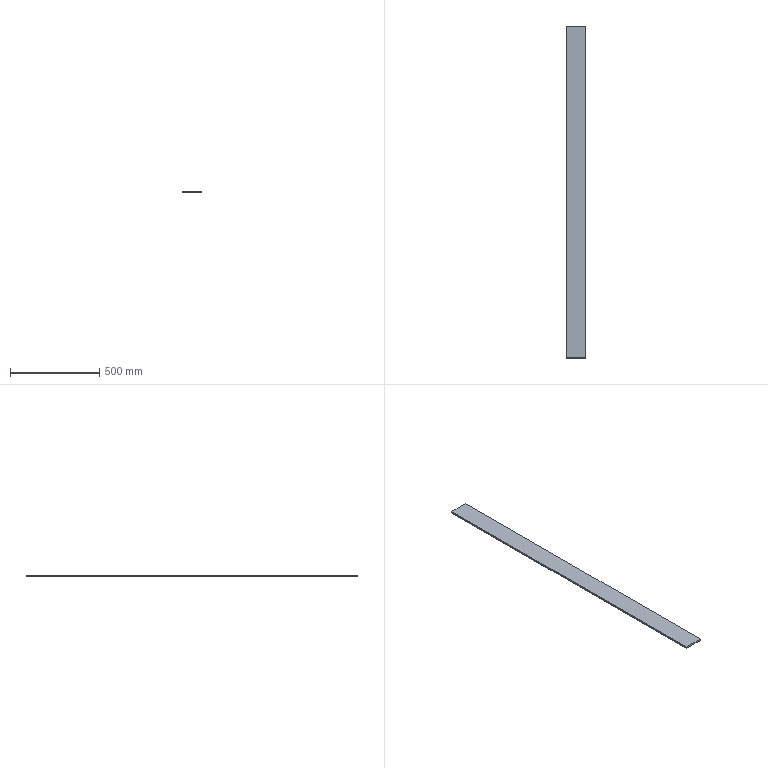Part | STEP file | 02-Steel plate | 1 solid | 6 faces | box 110 x 1860 x 10 mm | volume 2046000 mm3 | plane 6
STEP:
#1=CARTESIAN_POINT('',(0.,0.,0.));
#2=DIRECTION('',(0.,0.,1.));
#3=DIRECTION('',(1.,0.,0.));
#4=AXIS2_PLACEMENT_3D('',#1,#2,#3);
#5=CARTESIAN_POINT('',(0.,0.,0.));
#6=VERTEX_POINT('',#5);
#7=CARTESIAN_POINT('',(0.,-1860.,0.));
#8=VERTEX_POINT('',#7);
#9=CARTESIAN_POINT('',(0.,0.,0.));
#10=DIRECTION('',(0.,-1.,0.));
#11=VECTOR('',#10,1.);
#12=LINE('',#9,#11);
#13=CARTESIAN_POINT('',(0.,0.,10.));
#14=DIRECTION('',(1.,0.,0.));
#15=DIRECTION('',(0.,1.,0.));
#16=AXIS2_PLACEMENT_3D('',#13,#14,#15);
#17=PLANE('',#16);
#18=CARTESIAN_POINT('',(0.,-10.));
#19=DIRECTION('',(-1.,0.));
#20=VECTOR('',#19,1.);
#21=LINE('',#18,#20);
#22=(GEOMETRIC_REPRESENTATION_CONTEXT(2)PARAMETRIC_REPRESENTATION_CONTEXT()REPRESENTATION_CONTEXT('',''));
#23=DEFINITIONAL_REPRESENTATION('',(#21),#22);
#24=PCURVE('',#17,#23);
#25=CARTESIAN_POINT('',(0.,0.,0.));
#26=DIRECTION('',(0.,0.,1.));
#27=DIRECTION('',(1.,0.,0.));
#28=AXIS2_PLACEMENT_3D('',#25,#26,#27);
#29=PLANE('',#28);
#30=CARTESIAN_POINT('',(0.,0.));
#31=DIRECTION('',(0.,-1.));
#32=VECTOR('',#31,1.);
#33=LINE('',#30,#32);
#34=(GEOMETRIC_REPRESENTATION_CONTEXT(2)PARAMETRIC_REPRESENTATION_CONTEXT()REPRESENTATION_CONTEXT('',''));
#35=DEFINITIONAL_REPRESENTATION('',(#33),#34);
#36=PCURVE('',#29,#35);
#37=SURFACE_CURVE('',#12,(#24,#36),.PCURVE_S1.);
#38=EDGE_CURVE('',#6,#8,#37,.T.);
#39=ORIENTED_EDGE('',*,*,#38,.T.);
#40=CARTESIAN_POINT('',(0.,-1860.,10.));
#41=VERTEX_POINT('',#40);
#42=CARTESIAN_POINT('',(0.,-1860.,10.));
#43=DIRECTION('',(0.,0.,-1.));
#44=VECTOR('',#43,1.);
#45=LINE('',#42,#44);
#46=CARTESIAN_POINT('',(-1860.,0.));
#47=DIRECTION('',(0.,-1.));
#48=VECTOR('',#47,1.);
#49=LINE('',#46,#48);
#50=(GEOMETRIC_REPRESENTATION_CONTEXT(2)PARAMETRIC_REPRESENTATION_CONTEXT()REPRESENTATION_CONTEXT('',''));
#51=DEFINITIONAL_REPRESENTATION('',(#49),#50);
#52=PCURVE('',#17,#51);
#53=CARTESIAN_POINT('',(0.,-1860.,10.));
#54=DIRECTION('',(0.,1.,0.));
#55=DIRECTION('',(0.,0.,1.));
#56=AXIS2_PLACEMENT_3D('',#53,#54,#55);
#57=PLANE('',#56);
#58=CARTESIAN_POINT('',(0.,0.));
#59=DIRECTION('',(-1.,0.));
#60=VECTOR('',#59,1.);
#61=LINE('',#58,#60);
#62=(GEOMETRIC_REPRESENTATION_CONTEXT(2)PARAMETRIC_REPRESENTATION_CONTEXT()REPRESENTATION_CONTEXT('',''));
#63=DEFINITIONAL_REPRESENTATION('',(#61),#62);
#64=PCURVE('',#57,#63);
#65=SURFACE_CURVE('',#45,(#52,#64),.PCURVE_S1.);
#66=EDGE_CURVE('',#41,#8,#65,.T.);
#67=ORIENTED_EDGE('',*,*,#66,.F.);
#68=CARTESIAN_POINT('',(0.,0.,10.));
#69=VERTEX_POINT('',#68);
#70=CARTESIAN_POINT('',(0.,0.,10.));
#71=DIRECTION('',(0.,-1.,0.));
#72=VECTOR('',#71,1.);
#73=LINE('',#70,#72);
#74=CARTESIAN_POINT('',(0.,0.));
#75=DIRECTION('',(-1.,0.));
#76=VECTOR('',#75,1.);
#77=LINE('',#74,#76);
#78=(GEOMETRIC_REPRESENTATION_CONTEXT(2)PARAMETRIC_REPRESENTATION_CONTEXT()REPRESENTATION_CONTEXT('',''));
#79=DEFINITIONAL_REPRESENTATION('',(#77),#78);
#80=PCURVE('',#17,#79);
#81=CARTESIAN_POINT('',(0.,0.,10.));
#82=DIRECTION('',(0.,0.,1.));
#83=DIRECTION('',(1.,0.,0.));
#84=AXIS2_PLACEMENT_3D('',#81,#82,#83);
#85=PLANE('',#84);
#86=CARTESIAN_POINT('',(0.,0.));
#87=DIRECTION('',(0.,-1.));
#88=VECTOR('',#87,1.);
#89=LINE('',#86,#88);
#90=(GEOMETRIC_REPRESENTATION_CONTEXT(2)PARAMETRIC_REPRESENTATION_CONTEXT()REPRESENTATION_CONTEXT('',''));
#91=DEFINITIONAL_REPRESENTATION('',(#89),#90);
#92=PCURVE('',#85,#91);
#93=SURFACE_CURVE('',#73,(#80,#92),.PCURVE_S1.);
#94=EDGE_CURVE('',#69,#41,#93,.T.);
#95=ORIENTED_EDGE('',*,*,#94,.F.);
#96=CARTESIAN_POINT('',(0.,0.,10.));
#97=DIRECTION('',(0.,0.,-1.));
#98=VECTOR('',#97,1.);
#99=LINE('',#96,#98);
#100=CARTESIAN_POINT('',(0.,0.));
#101=DIRECTION('',(0.,-1.));
#102=VECTOR('',#101,1.);
#103=LINE('',#100,#102);
#104=(GEOMETRIC_REPRESENTATION_CONTEXT(2)PARAMETRIC_REPRESENTATION_CONTEXT()REPRESENTATION_CONTEXT('',''));
#105=DEFINITIONAL_REPRESENTATION('',(#103),#104);
#106=PCURVE('',#17,#105);
#107=CARTESIAN_POINT('',(0.,0.,10.));
#108=DIRECTION('',(0.,-1.,0.));
#109=DIRECTION('',(0.,0.,-1.));
#110=AXIS2_PLACEMENT_3D('',#107,#108,#109);
#111=PLANE('',#110);
#112=CARTESIAN_POINT('',(0.,0.));
#113=DIRECTION('',(1.,0.));
#114=VECTOR('',#113,1.);
#115=LINE('',#112,#114);
#116=(GEOMETRIC_REPRESENTATION_CONTEXT(2)PARAMETRIC_REPRESENTATION_CONTEXT()REPRESENTATION_CONTEXT('',''));
#117=DEFINITIONAL_REPRESENTATION('',(#115),#116);
#118=PCURVE('',#111,#117);
#119=SURFACE_CURVE('',#99,(#106,#118),.PCURVE_S1.);
#120=EDGE_CURVE('',#69,#6,#119,.T.);
#121=ORIENTED_EDGE('',*,*,#120,.T.);
#122=EDGE_LOOP('',(#39,#67,#95,#121));
#123=FACE_BOUND('',#122,.T.);
#124=ADVANCED_FACE('',(#123),#17,.F.);
#125=CARTESIAN_POINT('',(110.,-1860.,0.));
#126=VERTEX_POINT('',#125);
#127=CARTESIAN_POINT('',(0.,-1860.,0.));
#128=DIRECTION('',(1.,0.,0.));
#129=VECTOR('',#128,1.);
#130=LINE('',#127,#129);
#131=CARTESIAN_POINT('',(-10.,0.));
#132=DIRECTION('',(0.,1.));
#133=VECTOR('',#132,1.);
#134=LINE('',#131,#133);
#135=(GEOMETRIC_REPRESENTATION_CONTEXT(2)PARAMETRIC_REPRESENTATION_CONTEXT()REPRESENTATION_CONTEXT('',''));
#136=DEFINITIONAL_REPRESENTATION('',(#134),#135);
#137=PCURVE('',#57,#136);
#138=CARTESIAN_POINT('',(0.,-1860.));
#139=DIRECTION('',(1.,0.));
#140=VECTOR('',#139,1.);
#141=LINE('',#138,#140);
#142=(GEOMETRIC_REPRESENTATION_CONTEXT(2)PARAMETRIC_REPRESENTATION_CONTEXT()REPRESENTATION_CONTEXT('',''));
#143=DEFINITIONAL_REPRESENTATION('',(#141),#142);
#144=PCURVE('',#29,#143);
#145=SURFACE_CURVE('',#130,(#137,#144),.PCURVE_S1.);
#146=EDGE_CURVE('',#8,#126,#145,.T.);
#147=ORIENTED_EDGE('',*,*,#146,.T.);
#148=CARTESIAN_POINT('',(110.,-1860.,10.));
#149=VERTEX_POINT('',#148);
#150=CARTESIAN_POINT('',(110.,-1860.,10.));
#151=DIRECTION('',(0.,0.,-1.));
#152=VECTOR('',#151,1.);
#153=LINE('',#150,#152);
#154=CARTESIAN_POINT('',(0.,110.));
#155=DIRECTION('',(-1.,0.));
#156=VECTOR('',#155,1.);
#157=LINE('',#154,#156);
#158=(GEOMETRIC_REPRESENTATION_CONTEXT(2)PARAMETRIC_REPRESENTATION_CONTEXT()REPRESENTATION_CONTEXT('',''));
#159=DEFINITIONAL_REPRESENTATION('',(#157),#158);
#160=PCURVE('',#57,#159);
#161=CARTESIAN_POINT('',(110.,0.,10.));
#162=DIRECTION('',(-1.,0.,0.));
#163=DIRECTION('',(0.,-1.,0.));
#164=AXIS2_PLACEMENT_3D('',#161,#162,#163);
#165=PLANE('',#164);
#166=CARTESIAN_POINT('',(1860.,0.));
#167=DIRECTION('',(0.,-1.));
#168=VECTOR('',#167,1.);
#169=LINE('',#166,#168);
#170=(GEOMETRIC_REPRESENTATION_CONTEXT(2)PARAMETRIC_REPRESENTATION_CONTEXT()REPRESENTATION_CONTEXT('',''));
#171=DEFINITIONAL_REPRESENTATION('',(#169),#170);
#172=PCURVE('',#165,#171);
#173=SURFACE_CURVE('',#153,(#160,#172),.PCURVE_S1.);
#174=EDGE_CURVE('',#149,#126,#173,.T.);
#175=ORIENTED_EDGE('',*,*,#174,.F.);
#176=CARTESIAN_POINT('',(0.,-1860.,10.));
#177=DIRECTION('',(1.,0.,0.));
#178=VECTOR('',#177,1.);
#179=LINE('',#176,#178);
#180=CARTESIAN_POINT('',(0.,0.));
#181=DIRECTION('',(0.,1.));
#182=VECTOR('',#181,1.);
#183=LINE('',#180,#182);
#184=(GEOMETRIC_REPRESENTATION_CONTEXT(2)PARAMETRIC_REPRESENTATION_CONTEXT()REPRESENTATION_CONTEXT('',''));
#185=DEFINITIONAL_REPRESENTATION('',(#183),#184);
#186=PCURVE('',#57,#185);
#187=CARTESIAN_POINT('',(0.,-1860.));
#188=DIRECTION('',(1.,0.));
#189=VECTOR('',#188,1.);
#190=LINE('',#187,#189);
#191=(GEOMETRIC_REPRESENTATION_CONTEXT(2)PARAMETRIC_REPRESENTATION_CONTEXT()REPRESENTATION_CONTEXT('',''));
#192=DEFINITIONAL_REPRESENTATION('',(#190),#191);
#193=PCURVE('',#85,#192);
#194=SURFACE_CURVE('',#179,(#186,#193),.PCURVE_S1.);
#195=EDGE_CURVE('',#41,#149,#194,.T.);
#196=ORIENTED_EDGE('',*,*,#195,.F.);
#197=ORIENTED_EDGE('',*,*,#66,.T.);
#198=EDGE_LOOP('',(#147,#175,#196,#197));
#199=FACE_BOUND('',#198,.T.);
#200=ADVANCED_FACE('',(#199),#57,.F.);
#201=CARTESIAN_POINT('',(110.,0.,0.));
#202=VERTEX_POINT('',#201);
#203=CARTESIAN_POINT('',(110.,0.,0.));
#204=DIRECTION('',(0.,1.,0.));
#205=VECTOR('',#204,1.);
#206=LINE('',#203,#205);
#207=CARTESIAN_POINT('',(0.,-10.));
#208=DIRECTION('',(-1.,0.));
#209=VECTOR('',#208,1.);
#210=LINE('',#207,#209);
#211=(GEOMETRIC_REPRESENTATION_CONTEXT(2)PARAMETRIC_REPRESENTATION_CONTEXT()REPRESENTATION_CONTEXT('',''));
#212=DEFINITIONAL_REPRESENTATION('',(#210),#211);
#213=PCURVE('',#165,#212);
#214=CARTESIAN_POINT('',(110.,0.));
#215=DIRECTION('',(0.,1.));
#216=VECTOR('',#215,1.);
#217=LINE('',#214,#216);
#218=(GEOMETRIC_REPRESENTATION_CONTEXT(2)PARAMETRIC_REPRESENTATION_CONTEXT()REPRESENTATION_CONTEXT('',''));
#219=DEFINITIONAL_REPRESENTATION('',(#217),#218);
#220=PCURVE('',#29,#219);
#221=SURFACE_CURVE('',#206,(#213,#220),.PCURVE_S1.);
#222=EDGE_CURVE('',#126,#202,#221,.T.);
#223=ORIENTED_EDGE('',*,*,#222,.T.);
#224=CARTESIAN_POINT('',(110.,0.,10.));
#225=VERTEX_POINT('',#224);
#226=CARTESIAN_POINT('',(110.,0.,10.));
#227=DIRECTION('',(0.,0.,-1.));
#228=VECTOR('',#227,1.);
#229=LINE('',#226,#228);
#230=CARTESIAN_POINT('',(0.,0.));
#231=DIRECTION('',(0.,-1.));
#232=VECTOR('',#231,1.);
#233=LINE('',#230,#232);
#234=(GEOMETRIC_REPRESENTATION_CONTEXT(2)PARAMETRIC_REPRESENTATION_CONTEXT()REPRESENTATION_CONTEXT('',''));
#235=DEFINITIONAL_REPRESENTATION('',(#233),#234);
#236=PCURVE('',#165,#235);
#237=CARTESIAN_POINT('',(0.,110.));
#238=DIRECTION('',(1.,0.));
#239=VECTOR('',#238,1.);
#240=LINE('',#237,#239);
#241=(GEOMETRIC_REPRESENTATION_CONTEXT(2)PARAMETRIC_REPRESENTATION_CONTEXT()REPRESENTATION_CONTEXT('',''));
#242=DEFINITIONAL_REPRESENTATION('',(#240),#241);
#243=PCURVE('',#111,#242);
#244=SURFACE_CURVE('',#229,(#236,#243),.PCURVE_S1.);
#245=EDGE_CURVE('',#225,#202,#244,.T.);
#246=ORIENTED_EDGE('',*,*,#245,.F.);
#247=CARTESIAN_POINT('',(110.,0.,10.));
#248=DIRECTION('',(0.,1.,0.));
#249=VECTOR('',#248,1.);
#250=LINE('',#247,#249);
#251=CARTESIAN_POINT('',(0.,0.));
#252=DIRECTION('',(-1.,0.));
#253=VECTOR('',#252,1.);
#254=LINE('',#251,#253);
#255=(GEOMETRIC_REPRESENTATION_CONTEXT(2)PARAMETRIC_REPRESENTATION_CONTEXT()REPRESENTATION_CONTEXT('',''));
#256=DEFINITIONAL_REPRESENTATION('',(#254),#255);
#257=PCURVE('',#165,#256);
#258=CARTESIAN_POINT('',(110.,0.));
#259=DIRECTION('',(0.,1.));
#260=VECTOR('',#259,1.);
#261=LINE('',#258,#260);
#262=(GEOMETRIC_REPRESENTATION_CONTEXT(2)PARAMETRIC_REPRESENTATION_CONTEXT()REPRESENTATION_CONTEXT('',''));
#263=DEFINITIONAL_REPRESENTATION('',(#261),#262);
#264=PCURVE('',#85,#263);
#265=SURFACE_CURVE('',#250,(#257,#264),.PCURVE_S1.);
#266=EDGE_CURVE('',#149,#225,#265,.T.);
#267=ORIENTED_EDGE('',*,*,#266,.F.);
#268=ORIENTED_EDGE('',*,*,#174,.T.);
#269=EDGE_LOOP('',(#223,#246,#267,#268));
#270=FACE_BOUND('',#269,.T.);
#271=ADVANCED_FACE('',(#270),#165,.F.);
#272=CARTESIAN_POINT('',(0.,0.,0.));
#273=DIRECTION('',(-1.,0.,0.));
#274=VECTOR('',#273,1.);
#275=LINE('',#272,#274);
#276=CARTESIAN_POINT('',(10.,0.));
#277=DIRECTION('',(0.,-1.));
#278=VECTOR('',#277,1.);
#279=LINE('',#276,#278);
#280=(GEOMETRIC_REPRESENTATION_CONTEXT(2)PARAMETRIC_REPRESENTATION_CONTEXT()REPRESENTATION_CONTEXT('',''));
#281=DEFINITIONAL_REPRESENTATION('',(#279),#280);
#282=PCURVE('',#111,#281);
#283=CARTESIAN_POINT('',(0.,0.));
#284=DIRECTION('',(-1.,0.));
#285=VECTOR('',#284,1.);
#286=LINE('',#283,#285);
#287=(GEOMETRIC_REPRESENTATION_CONTEXT(2)PARAMETRIC_REPRESENTATION_CONTEXT()REPRESENTATION_CONTEXT('',''));
#288=DEFINITIONAL_REPRESENTATION('',(#286),#287);
#289=PCURVE('',#29,#288);
#290=SURFACE_CURVE('',#275,(#282,#289),.PCURVE_S1.);
#291=EDGE_CURVE('',#202,#6,#290,.T.);
#292=ORIENTED_EDGE('',*,*,#291,.T.);
#293=ORIENTED_EDGE('',*,*,#120,.F.);
#294=CARTESIAN_POINT('',(0.,0.,10.));
#295=DIRECTION('',(-1.,0.,0.));
#296=VECTOR('',#295,1.);
#297=LINE('',#294,#296);
#298=CARTESIAN_POINT('',(0.,0.));
#299=DIRECTION('',(0.,-1.));
#300=VECTOR('',#299,1.);
#301=LINE('',#298,#300);
#302=(GEOMETRIC_REPRESENTATION_CONTEXT(2)PARAMETRIC_REPRESENTATION_CONTEXT()REPRESENTATION_CONTEXT('',''));
#303=DEFINITIONAL_REPRESENTATION('',(#301),#302);
#304=PCURVE('',#111,#303);
#305=CARTESIAN_POINT('',(0.,0.));
#306=DIRECTION('',(-1.,0.));
#307=VECTOR('',#306,1.);
#308=LINE('',#305,#307);
#309=(GEOMETRIC_REPRESENTATION_CONTEXT(2)PARAMETRIC_REPRESENTATION_CONTEXT()REPRESENTATION_CONTEXT('',''));
#310=DEFINITIONAL_REPRESENTATION('',(#308),#309);
#311=PCURVE('',#85,#310);
#312=SURFACE_CURVE('',#297,(#304,#311),.PCURVE_S1.);
#313=EDGE_CURVE('',#225,#69,#312,.T.);
#314=ORIENTED_EDGE('',*,*,#313,.F.);
#315=ORIENTED_EDGE('',*,*,#245,.T.);
#316=EDGE_LOOP('',(#292,#293,#314,#315));
#317=FACE_BOUND('',#316,.T.);
#318=ADVANCED_FACE('',(#317),#111,.F.);
#319=ORIENTED_EDGE('',*,*,#94,.T.);
#320=ORIENTED_EDGE('',*,*,#195,.T.);
#321=ORIENTED_EDGE('',*,*,#266,.T.);
#322=ORIENTED_EDGE('',*,*,#313,.T.);
#323=EDGE_LOOP('',(#319,#320,#321,#322));
#324=FACE_BOUND('',#323,.T.);
#325=ADVANCED_FACE('',(#324),#85,.T.);
#326=ORIENTED_EDGE('',*,*,#38,.F.);
#327=ORIENTED_EDGE('',*,*,#291,.F.);
#328=ORIENTED_EDGE('',*,*,#222,.F.);
#329=ORIENTED_EDGE('',*,*,#146,.F.);
#330=EDGE_LOOP('',(#326,#327,#328,#329));
#331=FACE_BOUND('',#330,.T.);
#332=ADVANCED_FACE('',(#331),#29,.F.);
#333=CLOSED_SHELL('',(#124,#200,#271,#318,#325,#332));
#334=MANIFOLD_SOLID_BREP('',#333);
#335=(LENGTH_UNIT()NAMED_UNIT(*)SI_UNIT(.MILLI.,.METRE.));
#336=UNCERTAINTY_MEASURE_WITH_UNIT(LENGTH_MEASURE(0.0000001),#335,'','');
#337=(NAMED_UNIT(*)PLANE_ANGLE_UNIT()SI_UNIT($,.RADIAN.));
#338=(NAMED_UNIT(*)SI_UNIT($,.STERADIAN.)SOLID_ANGLE_UNIT());
#339=(GEOMETRIC_REPRESENTATION_CONTEXT(3)GLOBAL_UNCERTAINTY_ASSIGNED_CONTEXT((#336))GLOBAL_UNIT_ASSIGNED_CONTEXT((#335,#337,#338))REPRESENTATION_CONTEXT('',''));
#340=ADVANCED_BREP_SHAPE_REPRESENTATION('',(#4,#334),#339);